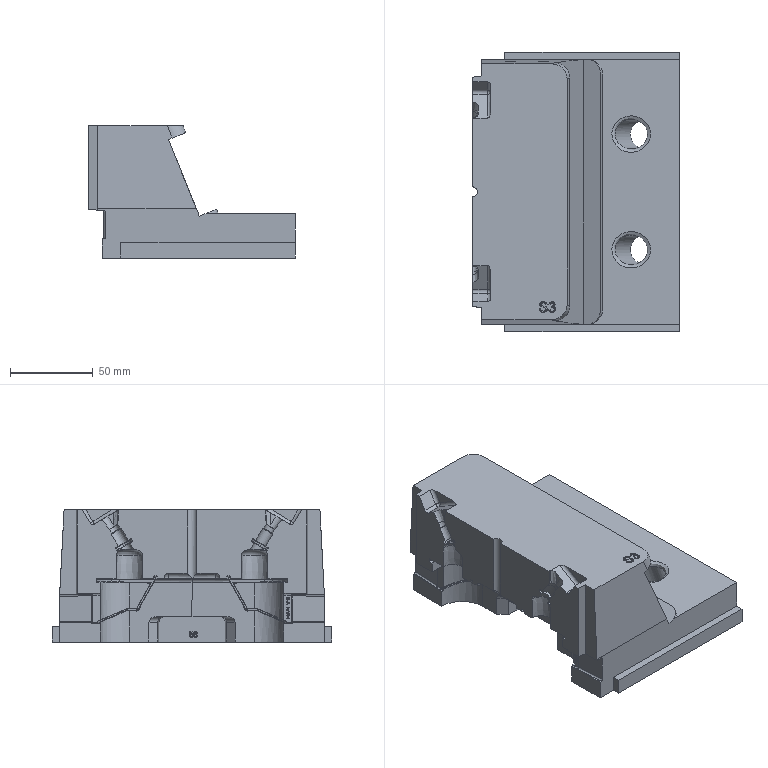Part | STEP file | lll_id90_x_t | 1 solid | 428 faces | box 125 x 169 x 80 mm | volume 846021 mm3 | plane 185 | cylinder 80 | spline 71 | other 68 | torus 10 | cone 10 | sphere 4 | commonest cylinder face diameters 6 x18 0.602 x14 2.008 x6 4 x6 18 x6 2 x4